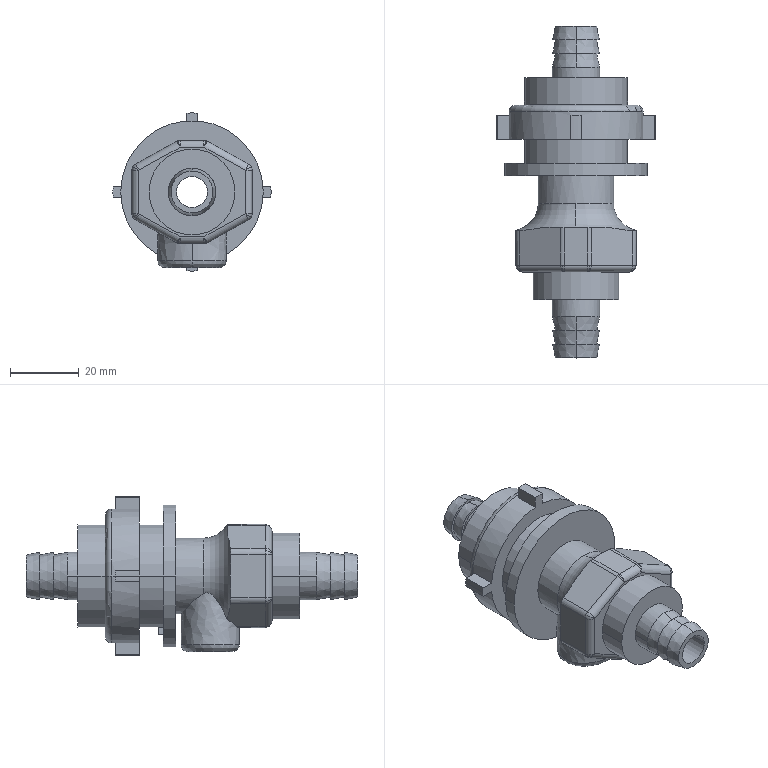Part | STEP file | 0D5CPC.stp.STEP | 1 solid | 115 faces | box 46 x 96.6 x 46 mm | volume 49865 mm3 | cylinder 41 | plane 38 | sphere 16 | cone 12 | torus 4 | spline 4 | commonest cylinder face diameters 4 x16 46 x5 13.8 x4 22 x4 30 x4 9 x2